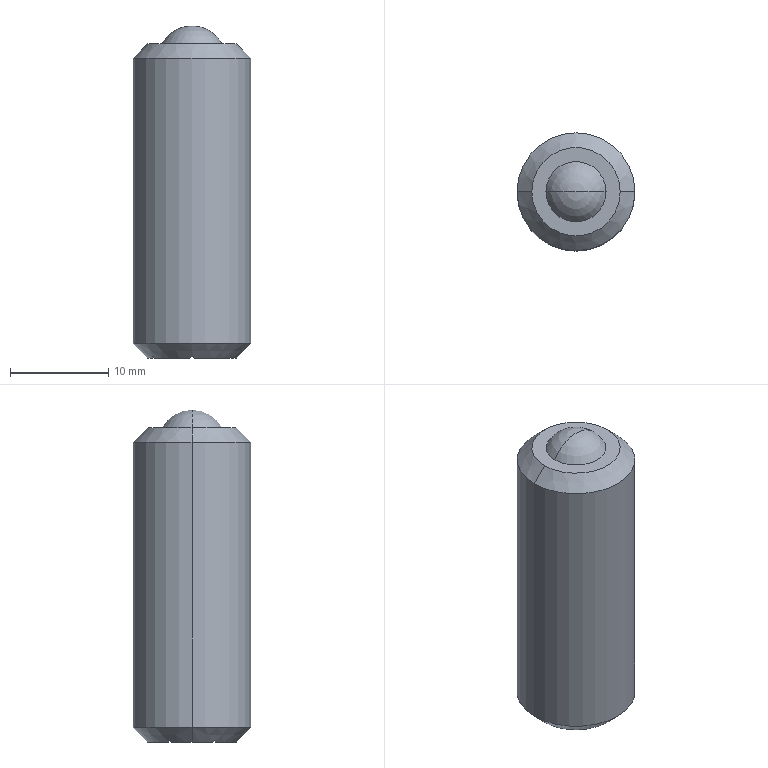Part | Creo | 1 solid | 22 faces | box 12 x 12 x 33.8 mm | volume 2573 mm3 | plane 14 | cone 4 | cylinder 2 | sphere 2 | commonest cylinder face diameters 12 x2
STEP:
#1=CARTESIAN_POINT('',(99.,-277.938,-72.5));
#2=VERTEX_POINT('',#1);
#3=CARTESIAN_POINT('',(99.,-282.062,-72.5));
#4=VERTEX_POINT('',#3);
#5=CARTESIAN_POINT('',(99.,-277.938,-72.5));
#6=DIRECTION('',(0.,-1.,0.));
#7=VECTOR('',#6,4.123);
#8=LINE('',#5,#7);
#9=EDGE_CURVE('',#2,#4,#8,.T.);
#10=ORIENTED_EDGE('',*,*,#9,.T.);
#11=CARTESIAN_POINT('',(99.5,-280.,-72.5));
#12=VERTEX_POINT('',#11);
#13=CARTESIAN_POINT('',(95.,-280.,-72.5));
#14=DIRECTION('',(0.,0.,-1.));
#15=DIRECTION('',(1.,0.,0.));
#16=AXIS2_PLACEMENT_3D('',#13,#14,#15);
#17=CIRCLE('',#16,4.5);
#18=EDGE_CURVE('',#12,#4,#17,.T.);
#19=ORIENTED_EDGE('',*,*,#18,.F.);
#20=CARTESIAN_POINT('',(95.,-280.,-72.5));
#21=DIRECTION('',(0.,0.,-1.));
#22=DIRECTION('',(0.8889,0.4581,0.));
#23=AXIS2_PLACEMENT_3D('',#20,#21,#22);
#24=CIRCLE('',#23,4.5);
#25=EDGE_CURVE('',#2,#12,#24,.T.);
#26=ORIENTED_EDGE('',*,*,#25,.F.);
#27=EDGE_LOOP('',(#10,#19,#26));
#28=FACE_OUTER_BOUND('',#27,.F.);
#29=CARTESIAN_POINT('',(95.,-280.,-72.5));
#30=DIRECTION('',(0.,0.,-1.));
#31=DIRECTION('',(-1.,0.,0.));
#32=AXIS2_PLACEMENT_3D('',#29,#30,#31);
#33=PLANE('',#32);
#34=ADVANCED_FACE('',(#28),#33,.T.);
#35=ORIENTED_EDGE('',*,*,#9,.F.);
#36=CARTESIAN_POINT('',(99.,-277.691,-72.381));
#37=VERTEX_POINT('',#36);
#38=CARTESIAN_POINT('',(99.,-277.938,-72.5));
#39=CARTESIAN_POINT('',(99.,-277.911,-72.487));
#40=CARTESIAN_POINT('',(99.,-277.856,-72.462));
#41=CARTESIAN_POINT('',(99.,-277.773,-72.422));
#42=CARTESIAN_POINT('',(99.,-277.718,-72.395));
#43=CARTESIAN_POINT('',(99.,-277.691,-72.381));
#44=B_SPLINE_CURVE_WITH_KNOTS('',3,(#38,#39,#40,#41,#42,#43),.UNSPECIFIED.,.F.,.F.,(4,1,1,4),(0.,0.3333,0.6667,1.),.UNSPECIFIED.);
#45=EDGE_CURVE('',#2,#37,#44,.T.);
#46=ORIENTED_EDGE('',*,*,#45,.T.);
#47=CARTESIAN_POINT('',(99.,-277.691,-54.5));
#48=VERTEX_POINT('',#47);
#49=CARTESIAN_POINT('',(99.,-277.691,-54.5));
#50=DIRECTION('',(0.,0.,-1.));
#51=VECTOR('',#50,17.881);
#52=LINE('',#49,#51);
#53=EDGE_CURVE('',#48,#37,#52,.T.);
#54=ORIENTED_EDGE('',*,*,#53,.F.);
#55=CARTESIAN_POINT('',(99.,-282.309,-54.5));
#56=VERTEX_POINT('',#55);
#57=CARTESIAN_POINT('',(99.,-277.691,-54.5));
#58=DIRECTION('',(0.,-1.,0.));
#59=VECTOR('',#58,4.619);
#60=LINE('',#57,#59);
#61=EDGE_CURVE('',#48,#56,#60,.T.);
#62=ORIENTED_EDGE('',*,*,#61,.T.);
#63=CARTESIAN_POINT('',(99.,-282.309,-72.381));
#64=VERTEX_POINT('',#63);
#65=CARTESIAN_POINT('',(99.,-282.309,-54.5));
#66=DIRECTION('',(0.,0.,-1.));
#67=VECTOR('',#66,17.881);
#68=LINE('',#65,#67);
#69=EDGE_CURVE('',#56,#64,#68,.T.);
#70=ORIENTED_EDGE('',*,*,#69,.T.);
#71=CARTESIAN_POINT('',(99.,-282.309,-72.381));
#72=CARTESIAN_POINT('',(99.,-282.282,-72.395));
#73=CARTESIAN_POINT('',(99.,-282.227,-72.422));
#74=CARTESIAN_POINT('',(99.,-282.144,-72.462));
#75=CARTESIAN_POINT('',(99.,-282.089,-72.487));
#76=CARTESIAN_POINT('',(99.,-282.062,-72.5));
#77=B_SPLINE_CURVE_WITH_KNOTS('',3,(#71,#72,#73,#74,#75,#76),.UNSPECIFIED.,.F.,.F.,(4,1,1,4),(0.,0.3333,0.6667,1.),.UNSPECIFIED.);
#78=EDGE_CURVE('',#64,#4,#77,.T.);
#79=ORIENTED_EDGE('',*,*,#78,.T.);
#80=EDGE_LOOP('',(#35,#46,#54,#62,#70,#79));
#81=FACE_OUTER_BOUND('',#80,.F.);
#82=CARTESIAN_POINT('',(99.,-280.,-68.5));
#83=DIRECTION('',(1.,0.,0.));
#84=DIRECTION('',(0.,0.,-1.));
#85=AXIS2_PLACEMENT_3D('',#82,#83,#84);
#86=PLANE('',#85);
#87=ADVANCED_FACE('',(#81),#86,.F.);
#88=ORIENTED_EDGE('',*,*,#25,.T.);
#89=CARTESIAN_POINT('',(101.,-280.,-71.));
#90=VERTEX_POINT('',#89);
#91=CARTESIAN_POINT('',(99.5,-280.,-72.5));
#92=DIRECTION('',(0.7071,0.,0.7071));
#93=VECTOR('',#92,2.121);
#94=LINE('',#91,#93);
#95=EDGE_CURVE('',#12,#90,#94,.T.);
#96=ORIENTED_EDGE('',*,*,#95,.T.);
#97=CARTESIAN_POINT('',(89.,-280.,-71.));
#98=VERTEX_POINT('',#97);
#99=CARTESIAN_POINT('',(95.,-280.,-71.));
#100=DIRECTION('',(0.,0.,-1.));
#101=DIRECTION('',(-1.,0.,0.));
#102=AXIS2_PLACEMENT_3D('',#99,#100,#101);
#103=CIRCLE('',#102,6.);
#104=EDGE_CURVE('',#98,#90,#103,.T.);
#105=ORIENTED_EDGE('',*,*,#104,.F.);
#106=CARTESIAN_POINT('',(90.5,-280.,-72.5));
#107=VERTEX_POINT('',#106);
#108=CARTESIAN_POINT('',(90.5,-280.,-72.5));
#109=DIRECTION('',(-0.7071,0.,0.7071));
#110=VECTOR('',#109,2.121);
#111=LINE('',#108,#110);
#112=EDGE_CURVE('',#107,#98,#111,.T.);
#113=ORIENTED_EDGE('',*,*,#112,.F.);
#114=CARTESIAN_POINT('',(91.,-277.938,-72.5));
#115=VERTEX_POINT('',#114);
#116=CARTESIAN_POINT('',(95.,-280.,-72.5));
#117=DIRECTION('',(0.,0.,-1.));
#118=DIRECTION('',(-1.,0.,0.));
#119=AXIS2_PLACEMENT_3D('',#116,#117,#118);
#120=CIRCLE('',#119,4.5);
#121=EDGE_CURVE('',#107,#115,#120,.T.);
#122=ORIENTED_EDGE('',*,*,#121,.T.);
#123=CARTESIAN_POINT('',(91.,-277.691,-72.381));
#124=VERTEX_POINT('',#123);
#125=CARTESIAN_POINT('',(91.,-277.691,-72.381));
#126=CARTESIAN_POINT('',(91.,-277.718,-72.395));
#127=CARTESIAN_POINT('',(91.,-277.773,-72.422));
#128=CARTESIAN_POINT('',(91.,-277.856,-72.462));
#129=CARTESIAN_POINT('',(91.,-277.911,-72.487));
#130=CARTESIAN_POINT('',(91.,-277.938,-72.5));
#131=B_SPLINE_CURVE_WITH_KNOTS('',3,(#125,#126,#127,#128,#129,#130),.UNSPECIFIED.,.F.,.F.,(4,1,1,4),(0.,0.3333,0.6667,1.),.UNSPECIFIED.);
#132=EDGE_CURVE('',#124,#115,#131,.T.);
#133=ORIENTED_EDGE('',*,*,#132,.F.);
#134=CARTESIAN_POINT('',(91.215,-277.567,-72.5));
#135=VERTEX_POINT('',#134);
#136=CARTESIAN_POINT('',(91.215,-277.567,-72.5));
#137=CARTESIAN_POINT('',(91.191,-277.58,-72.487));
#138=CARTESIAN_POINT('',(91.143,-277.608,-72.462));
#139=CARTESIAN_POINT('',(91.071,-277.649,-72.422));
#140=CARTESIAN_POINT('',(91.024,-277.677,-72.395));
#141=CARTESIAN_POINT('',(91.,-277.691,-72.381));
#142=B_SPLINE_CURVE_WITH_KNOTS('',3,(#136,#137,#138,#139,#140,#141),.UNSPECIFIED.,.F.,.F.,(4,1,1,4),(0.,0.3333,0.6667,1.),.UNSPECIFIED.);
#143=EDGE_CURVE('',#135,#124,#142,.T.);
#144=ORIENTED_EDGE('',*,*,#143,.F.);
#145=CARTESIAN_POINT('',(94.785,-275.505,-72.5));
#146=VERTEX_POINT('',#145);
#147=CARTESIAN_POINT('',(95.,-280.,-72.5));
#148=DIRECTION('',(0.,0.,-1.));
#149=DIRECTION('',(-0.8412,0.5407,0.));
#150=AXIS2_PLACEMENT_3D('',#147,#148,#149);
#151=CIRCLE('',#150,4.5);
#152=EDGE_CURVE('',#135,#146,#151,.T.);
#153=ORIENTED_EDGE('',*,*,#152,.T.);
#154=CARTESIAN_POINT('',(95.,-275.381,-72.381));
#155=VERTEX_POINT('',#154);
#156=CARTESIAN_POINT('',(95.,-275.381,-72.381));
#157=CARTESIAN_POINT('',(94.976,-275.395,-72.395));
#158=CARTESIAN_POINT('',(94.929,-275.422,-72.422));
#159=CARTESIAN_POINT('',(94.857,-275.464,-72.462));
#160=CARTESIAN_POINT('',(94.809,-275.491,-72.487));
#161=CARTESIAN_POINT('',(94.785,-275.505,-72.5));
#162=B_SPLINE_CURVE_WITH_KNOTS('',3,(#156,#157,#158,#159,#160,#161),.UNSPECIFIED.,.F.,.F.,(4,1,1,4),(0.,0.3333,0.6667,1.),.UNSPECIFIED.);
#163=EDGE_CURVE('',#155,#146,#162,.T.);
#164=ORIENTED_EDGE('',*,*,#163,.F.);
#165=CARTESIAN_POINT('',(95.215,-275.505,-72.5));
#166=VERTEX_POINT('',#165);
#167=CARTESIAN_POINT('',(95.215,-275.505,-72.5));
#168=CARTESIAN_POINT('',(95.191,-275.491,-72.487));
#169=CARTESIAN_POINT('',(95.143,-275.464,-72.462));
#170=CARTESIAN_POINT('',(95.071,-275.422,-72.422));
#171=CARTESIAN_POINT('',(95.024,-275.395,-72.395));
#172=CARTESIAN_POINT('',(95.,-275.381,-72.381));
#173=B_SPLINE_CURVE_WITH_KNOTS('',3,(#167,#168,#169,#170,#171,#172),.UNSPECIFIED.,.F.,.F.,(4,1,1,4),(0.,0.3333,0.6667,1.),.UNSPECIFIED.);
#174=EDGE_CURVE('',#166,#155,#173,.T.);
#175=ORIENTED_EDGE('',*,*,#174,.F.);
#176=CARTESIAN_POINT('',(98.785,-277.567,-72.5));
#177=VERTEX_POINT('',#176);
#178=CARTESIAN_POINT('',(95.,-280.,-72.5));
#179=DIRECTION('',(0.,0.,-1.));
#180=DIRECTION('',(0.0477,0.9989,0.));
#181=AXIS2_PLACEMENT_3D('',#178,#179,#180);
#182=CIRCLE('',#181,4.5);
#183=EDGE_CURVE('',#166,#177,#182,.T.);
#184=ORIENTED_EDGE('',*,*,#183,.T.);
#185=CARTESIAN_POINT('',(99.,-277.691,-72.381));
#186=CARTESIAN_POINT('',(98.976,-277.677,-72.395));
#187=CARTESIAN_POINT('',(98.929,-277.649,-72.422));
#188=CARTESIAN_POINT('',(98.857,-277.608,-72.462));
#189=CARTESIAN_POINT('',(98.809,-277.58,-72.487));
#190=CARTESIAN_POINT('',(98.785,-277.567,-72.5));
#191=B_SPLINE_CURVE_WITH_KNOTS('',3,(#185,#186,#187,#188,#189,#190),.UNSPECIFIED.,.F.,.F.,(4,1,1,4),(0.,0.3333,0.6667,1.),.UNSPECIFIED.);
#192=EDGE_CURVE('',#37,#177,#191,.T.);
#193=ORIENTED_EDGE('',*,*,#192,.F.);
#194=ORIENTED_EDGE('',*,*,#45,.F.);
#195=EDGE_LOOP('',(#88,#96,#105,#113,#122,#133,#144,#153,#164,#175,#184,#193,#194));
#196=FACE_OUTER_BOUND('',#195,.F.);
#197=CARTESIAN_POINT('',(95.,-280.,-71.75));
#198=DIRECTION('',(0.,0.,1.));
#199=DIRECTION('',(1.,0.,0.));
#200=AXIS2_PLACEMENT_3D('',#197,#198,#199);
#201=CONICAL_SURFACE('',#200,5.25,45.);
#202=ADVANCED_FACE('',(#196),#201,.T.);
#203=ORIENTED_EDGE('',*,*,#78,.F.);
#204=CARTESIAN_POINT('',(98.785,-282.433,-72.5));
#205=VERTEX_POINT('',#204);
#206=CARTESIAN_POINT('',(98.785,-282.433,-72.5));
#207=CARTESIAN_POINT('',(98.809,-282.42,-72.487));
#208=CARTESIAN_POINT('',(98.857,-282.392,-72.462));
#209=CARTESIAN_POINT('',(98.929,-282.351,-72.422));
#210=CARTESIAN_POINT('',(98.976,-282.323,-72.395));
#211=CARTESIAN_POINT('',(99.,-282.309,-72.381));
#212=B_SPLINE_CURVE_WITH_KNOTS('',3,(#206,#207,#208,#209,#210,#211),.UNSPECIFIED.,.F.,.F.,(4,1,1,4),(0.,0.3333,0.6667,1.),.UNSPECIFIED.);
#213=EDGE_CURVE('',#205,#64,#212,.T.);
#214=ORIENTED_EDGE('',*,*,#213,.F.);
#215=CARTESIAN_POINT('',(95.215,-284.495,-72.5));
#216=VERTEX_POINT('',#215);
#217=CARTESIAN_POINT('',(95.,-280.,-72.5));
#218=DIRECTION('',(0.,0.,-1.));
#219=DIRECTION('',(0.8412,-0.5407,0.));
#220=AXIS2_PLACEMENT_3D('',#217,#218,#219);
#221=CIRCLE('',#220,4.5);
#222=EDGE_CURVE('',#205,#216,#221,.T.);
#223=ORIENTED_EDGE('',*,*,#222,.T.);
#224=CARTESIAN_POINT('',(95.,-284.619,-72.381));
#225=VERTEX_POINT('',#224);
#226=CARTESIAN_POINT('',(95.,-284.619,-72.381));
#227=CARTESIAN_POINT('',(95.024,-284.605,-72.395));
#228=CARTESIAN_POINT('',(95.071,-284.578,-72.422));
#229=CARTESIAN_POINT('',(95.143,-284.536,-72.462));
#230=CARTESIAN_POINT('',(95.191,-284.509,-72.487));
#231=CARTESIAN_POINT('',(95.215,-284.495,-72.5));
#232=B_SPLINE_CURVE_WITH_KNOTS('',3,(#226,#227,#228,#229,#230,#231),.UNSPECIFIED.,.F.,.F.,(4,1,1,4),(0.,0.3333,0.6667,1.),.UNSPECIFIED.);
#233=EDGE_CURVE('',#225,#216,#232,.T.);
#234=ORIENTED_EDGE('',*,*,#233,.F.);
#235=CARTESIAN_POINT('',(94.785,-284.495,-72.5));
#236=VERTEX_POINT('',#235);
#237=CARTESIAN_POINT('',(94.785,-284.495,-72.5));
#238=CARTESIAN_POINT('',(94.809,-284.509,-72.487));
#239=CARTESIAN_POINT('',(94.857,-284.536,-72.462));
#240=CARTESIAN_POINT('',(94.929,-284.578,-72.422));
#241=CARTESIAN_POINT('',(94.976,-284.605,-72.395));
#242=CARTESIAN_POINT('',(95.,-284.619,-72.381));
#243=B_SPLINE_CURVE_WITH_KNOTS('',3,(#237,#238,#239,#240,#241,#242),.UNSPECIFIED.,.F.,.F.,(4,1,1,4),(0.,0.3333,0.6667,1.),.UNSPECIFIED.);
#244=EDGE_CURVE('',#236,#225,#243,.T.);
#245=ORIENTED_EDGE('',*,*,#244,.F.);
#246=CARTESIAN_POINT('',(91.215,-282.433,-72.5));
#247=VERTEX_POINT('',#246);
#248=CARTESIAN_POINT('',(95.,-280.,-72.5));
#249=DIRECTION('',(0.,0.,-1.));
#250=DIRECTION('',(-0.0477,-0.9989,0.));
#251=AXIS2_PLACEMENT_3D('',#248,#249,#250);
#252=CIRCLE('',#251,4.5);
#253=EDGE_CURVE('',#236,#247,#252,.T.);
#254=ORIENTED_EDGE('',*,*,#253,.T.);
#255=CARTESIAN_POINT('',(91.,-282.309,-72.381));
#256=VERTEX_POINT('',#255);
#257=CARTESIAN_POINT('',(91.,-282.309,-72.381));
#258=CARTESIAN_POINT('',(91.024,-282.323,-72.395));
#259=CARTESIAN_POINT('',(91.071,-282.351,-72.422));
#260=CARTESIAN_POINT('',(91.143,-282.392,-72.462));
#261=CARTESIAN_POINT('',(91.191,-282.42,-72.487));
#262=CARTESIAN_POINT('',(91.215,-282.433,-72.5));
#263=B_SPLINE_CURVE_WITH_KNOTS('',3,(#257,#258,#259,#260,#261,#262),.UNSPECIFIED.,.F.,.F.,(4,1,1,4),(0.,0.3333,0.6667,1.),.UNSPECIFIED.);
#264=EDGE_CURVE('',#256,#247,#263,.T.);
#265=ORIENTED_EDGE('',*,*,#264,.F.);
#266=CARTESIAN_POINT('',(91.,-282.062,-72.5));
#267=VERTEX_POINT('',#266);
#268=CARTESIAN_POINT('',(91.,-282.062,-72.5));
#269=CARTESIAN_POINT('',(91.,-282.089,-72.487));
#270=CARTESIAN_POINT('',(91.,-282.144,-72.462));
#271=CARTESIAN_POINT('',(91.,-282.227,-72.422));
#272=CARTESIAN_POINT('',(91.,-282.282,-72.395));
#273=CARTESIAN_POINT('',(91.,-282.309,-72.381));
#274=B_SPLINE_CURVE_WITH_KNOTS('',3,(#268,#269,#270,#271,#272,#273),.UNSPECIFIED.,.F.,.F.,(4,1,1,4),(0.,0.3333,0.6667,1.),.UNSPECIFIED.);
#275=EDGE_CURVE('',#267,#256,#274,.T.);
#276=ORIENTED_EDGE('',*,*,#275,.F.);
#277=CARTESIAN_POINT('',(95.,-280.,-72.5));
#278=DIRECTION('',(0.,0.,-1.));
#279=DIRECTION('',(-0.8889,-0.4581,0.));
#280=AXIS2_PLACEMENT_3D('',#277,#278,#279);
#281=CIRCLE('',#280,4.5);
#282=EDGE_CURVE('',#267,#107,#281,.T.);
#283=ORIENTED_EDGE('',*,*,#282,.T.);
#284=ORIENTED_EDGE('',*,*,#112,.T.);
#285=CARTESIAN_POINT('',(95.,-280.,-71.));
#286=DIRECTION('',(0.,0.,-1.));
#287=DIRECTION('',(1.,0.,0.));
#288=AXIS2_PLACEMENT_3D('',#285,#286,#287);
#289=CIRCLE('',#288,6.);
#290=EDGE_CURVE('',#90,#98,#289,.T.);
#291=ORIENTED_EDGE('',*,*,#290,.F.);
#292=ORIENTED_EDGE('',*,*,#95,.F.);
#293=ORIENTED_EDGE('',*,*,#18,.T.);
#294=EDGE_LOOP('',(#203,#214,#223,#234,#245,#254,#265,#276,#283,#284,#291,#292,#293));
#295=FACE_OUTER_BOUND('',#294,.F.);
#296=CARTESIAN_POINT('',(95.,-280.,-71.75));
#297=DIRECTION('',(0.,0.,1.));
#298=DIRECTION('',(1.,0.,0.));
#299=AXIS2_PLACEMENT_3D('',#296,#297,#298);
#300=CONICAL_SURFACE('',#299,5.25,45.);
#301=ADVANCED_FACE('',(#295),#300,.T.);
#302=ORIENTED_EDGE('',*,*,#69,.F.);
#303=CARTESIAN_POINT('',(95.,-284.619,-54.5));
#304=VERTEX_POINT('',#303);
#305=CARTESIAN_POINT('',(99.,-282.309,-54.5));
#306=DIRECTION('',(-0.866,-0.5,0.));
#307=VECTOR('',#306,4.619);
#308=LINE('',#305,#307);
#309=EDGE_CURVE('',#56,#304,#308,.T.);
#310=ORIENTED_EDGE('',*,*,#309,.T.);
#311=CARTESIAN_POINT('',(95.,-284.619,-54.5));
#312=DIRECTION('',(0.,0.,-1.));
#313=VECTOR('',#312,17.881);
#314=LINE('',#311,#313);
#315=EDGE_CURVE('',#304,#225,#314,.T.);
#316=ORIENTED_EDGE('',*,*,#315,.T.);
#317=ORIENTED_EDGE('',*,*,#233,.T.);
#318=CARTESIAN_POINT('',(95.215,-284.495,-72.5));
#319=DIRECTION('',(0.866,0.5,0.));
#320=VECTOR('',#319,4.123);
#321=LINE('',#318,#320);
#322=EDGE_CURVE('',#216,#205,#321,.T.);
#323=ORIENTED_EDGE('',*,*,#322,.T.);
#324=ORIENTED_EDGE('',*,*,#213,.T.);
#325=EDGE_LOOP('',(#302,#310,#316,#317,#323,#324));
#326=FACE_OUTER_BOUND('',#325,.F.);
#327=CARTESIAN_POINT('',(97.,-283.464,-68.5));
#328=DIRECTION('',(0.5,-0.866,0.));
#329=DIRECTION('',(0.866,0.5,0.));
#330=AXIS2_PLACEMENT_3D('',#327,#328,#329);
#331=PLANE('',#330);
#332=ADVANCED_FACE('',(#326),#331,.F.);
#333=CARTESIAN_POINT('',(91.,-282.309,-54.5));
#334=VERTEX_POINT('',#333);
#335=CARTESIAN_POINT('',(91.,-277.691,-54.5));
#336=VERTEX_POINT('',#335);
#337=CARTESIAN_POINT('',(91.,-282.309,-54.5));
#338=DIRECTION('',(0.,1.,0.));
#339=VECTOR('',#338,4.619);
#340=LINE('',#337,#339);
#341=EDGE_CURVE('',#334,#336,#340,.T.);
#342=ORIENTED_EDGE('',*,*,#341,.F.);
#343=CARTESIAN_POINT('',(95.,-284.619,-54.5));
#344=DIRECTION('',(-0.866,0.5,0.));
#345=VECTOR('',#344,4.619);
#346=LINE('',#343,#345);
#347=EDGE_CURVE('',#304,#334,#346,.T.);
#348=ORIENTED_EDGE('',*,*,#347,.F.);
#349=ORIENTED_EDGE('',*,*,#309,.F.);
#350=ORIENTED_EDGE('',*,*,#61,.F.);
#351=CARTESIAN_POINT('',(95.,-275.381,-54.5));
#352=VERTEX_POINT('',#351);
#353=CARTESIAN_POINT('',(95.,-275.381,-54.5));
#354=DIRECTION('',(0.866,-0.5,0.));
#355=VECTOR('',#354,4.619);
#356=LINE('',#353,#355);
#357=EDGE_CURVE('',#352,#48,#356,.T.);
#358=ORIENTED_EDGE('',*,*,#357,.F.);
#359=CARTESIAN_POINT('',(91.,-277.691,-54.5));
#360=DIRECTION('',(0.866,0.5,0.));
#361=VECTOR('',#360,4.619);
#362=LINE('',#359,#361);
#363=EDGE_CURVE('',#336,#352,#362,.T.);
#364=ORIENTED_EDGE('',*,*,#363,.F.);
#365=EDGE_LOOP('',(#342,#348,#349,#350,#358,#364));
#366=FACE_OUTER_BOUND('',#365,.F.);
#367=CARTESIAN_POINT('',(95.,-280.,-54.5));
#368=DIRECTION('',(0.,0.,1.));
#369=DIRECTION('',(1.,0.,0.));
#370=AXIS2_PLACEMENT_3D('',#367,#368,#369);
#371=PLANE('',#370);
#372=ADVANCED_FACE('',(#366),#371,.F.);
#373=CARTESIAN_POINT('',(91.,-282.309,-54.5));
#374=DIRECTION('',(0.,0.,-1.));
#375=VECTOR('',#374,17.881);
#376=LINE('',#373,#375);
#377=EDGE_CURVE('',#334,#256,#376,.T.);
#378=ORIENTED_EDGE('',*,*,#377,.F.);
#379=ORIENTED_EDGE('',*,*,#341,.T.);
#380=CARTESIAN_POINT('',(91.,-277.691,-54.5));
#381=DIRECTION('',(0.,0.,-1.));
#382=VECTOR('',#381,17.881);
#383=LINE('',#380,#382);
#384=EDGE_CURVE('',#336,#124,#383,.T.);
#385=ORIENTED_EDGE('',*,*,#384,.T.);
#386=ORIENTED_EDGE('',*,*,#132,.T.);
#387=CARTESIAN_POINT('',(91.,-282.062,-72.5));
#388=DIRECTION('',(0.,1.,0.));
#389=VECTOR('',#388,4.123);
#390=LINE('',#387,#389);
#391=EDGE_CURVE('',#267,#115,#390,.T.);
#392=ORIENTED_EDGE('',*,*,#391,.F.);
#393=ORIENTED_EDGE('',*,*,#275,.T.);
#394=EDGE_LOOP('',(#378,#379,#385,#386,#392,#393));
#395=FACE_OUTER_BOUND('',#394,.F.);
#396=CARTESIAN_POINT('',(91.,-280.,-68.5));
#397=DIRECTION('',(-1.,0.,0.));
#398=DIRECTION('',(0.,0.,1.));
#399=AXIS2_PLACEMENT_3D('',#396,#397,#398);
#400=PLANE('',#399);
#401=ADVANCED_FACE('',(#395),#400,.F.);
#402=ORIENTED_EDGE('',*,*,#315,.F.);
#403=ORIENTED_EDGE('',*,*,#347,.T.);
#404=ORIENTED_EDGE('',*,*,#377,.T.);
#405=ORIENTED_EDGE('',*,*,#264,.T.);
#406=CARTESIAN_POINT('',(91.215,-282.433,-72.5));
#407=DIRECTION('',(0.866,-0.5,0.));
#408=VECTOR('',#407,4.123);
#409=LINE('',#406,#408);
#410=EDGE_CURVE('',#247,#236,#409,.T.);
#411=ORIENTED_EDGE('',*,*,#410,.T.);
#412=ORIENTED_EDGE('',*,*,#244,.T.);
#413=EDGE_LOOP('',(#402,#403,#404,#405,#411,#412));
#414=FACE_OUTER_BOUND('',#413,.F.);
#415=CARTESIAN_POINT('',(93.,-283.464,-68.5));
#416=DIRECTION('',(-0.5,-0.866,0.));
#417=DIRECTION('',(0.866,-0.5,0.));
#418=AXIS2_PLACEMENT_3D('',#415,#416,#417);
#419=PLANE('',#418);
#420=ADVANCED_FACE('',(#414),#419,.F.);
#421=ORIENTED_EDGE('',*,*,#410,.F.);
#422=ORIENTED_EDGE('',*,*,#253,.F.);
#423=EDGE_LOOP('',(#421,#422));
#424=FACE_OUTER_BOUND('',#423,.F.);
#425=CARTESIAN_POINT('',(75.,-280.,-72.5));
#426=DIRECTION('',(0.,0.,-1.));
#427=DIRECTION('',(-1.,0.,0.));
#428=AXIS2_PLACEMENT_3D('',#425,#426,#427);
#429=PLANE('',#428);
#430=ADVANCED_FACE('',(#424),#429,.T.);
#431=ORIENTED_EDGE('',*,*,#384,.F.);
#432=ORIENTED_EDGE('',*,*,#363,.T.);
#433=CARTESIAN_POINT('',(95.,-275.381,-54.5));
#434=DIRECTION('',(0.,0.,-1.));
#435=VECTOR('',#434,17.881);
#436=LINE('',#433,#435);
#437=EDGE_CURVE('',#352,#155,#436,.T.);
#438=ORIENTED_EDGE('',*,*,#437,.T.);
#439=ORIENTED_EDGE('',*,*,#163,.T.);
#440=CARTESIAN_POINT('',(94.785,-275.505,-72.5));
#441=DIRECTION('',(-0.866,-0.5,0.));
#442=VECTOR('',#441,4.123);
#443=LINE('',#440,#442);
#444=EDGE_CURVE('',#146,#135,#443,.T.);
#445=ORIENTED_EDGE('',*,*,#444,.T.);
#446=ORIENTED_EDGE('',*,*,#143,.T.);
#447=EDGE_LOOP('',(#431,#432,#438,#439,#445,#446));
#448=FACE_OUTER_BOUND('',#447,.F.);
#449=CARTESIAN_POINT('',(93.,-276.536,-68.5));
#450=DIRECTION('',(-0.5,0.866,0.));
#451=DIRECTION('',(-0.866,-0.5,0.));
#452=AXIS2_PLACEMENT_3D('',#449,#450,#451);
#453=PLANE('',#452);
#454=ADVANCED_FACE('',(#448),#453,.F.);
#455=ORIENTED_EDGE('',*,*,#437,.F.);
#456=ORIENTED_EDGE('',*,*,#357,.T.);
#457=ORIENTED_EDGE('',*,*,#53,.T.);
#458=ORIENTED_EDGE('',*,*,#192,.T.);
#459=CARTESIAN_POINT('',(98.785,-277.567,-72.5));
#460=DIRECTION('',(-0.866,0.5,0.));
#461=VECTOR('',#460,4.123);
#462=LINE('',#459,#461);
#463=EDGE_CURVE('',#177,#166,#462,.T.);
#464=ORIENTED_EDGE('',*,*,#463,.T.);
#465=ORIENTED_EDGE('',*,*,#174,.T.);
#466=EDGE_LOOP('',(#455,#456,#457,#458,#464,#465));
#467=FACE_OUTER_BOUND('',#466,.F.);
#468=CARTESIAN_POINT('',(97.,-276.536,-68.5));
#469=DIRECTION('',(0.5,0.866,0.));
#470=DIRECTION('',(-0.866,0.5,0.));
#471=AXIS2_PLACEMENT_3D('',#468,#469,#470);
#472=PLANE('',#471);
#473=ADVANCED_FACE('',(#467),#472,.F.);
#474=ORIENTED_EDGE('',*,*,#463,.F.);
#475=ORIENTED_EDGE('',*,*,#183,.F.);
#476=EDGE_LOOP('',(#474,#475));
#477=FACE_OUTER_BOUND('',#476,.F.);
#478=CARTESIAN_POINT('',(95.,-280.,-72.5));
#479=DIRECTION('',(0.,0.,-1.));
#480=DIRECTION('',(-1.,0.,0.));
#481=AXIS2_PLACEMENT_3D('',#478,#479,#480);
#482=PLANE('',#481);
#483=ADVANCED_FACE('',(#477),#482,.T.);
#484=ORIENTED_EDGE('',*,*,#444,.F.);
#485=ORIENTED_EDGE('',*,*,#152,.F.);
#486=EDGE_LOOP('',(#484,#485));
#487=FACE_OUTER_BOUND('',#486,.F.);
#488=CARTESIAN_POINT('',(95.,-280.,-72.5));
#489=DIRECTION('',(0.,0.,-1.));
#490=DIRECTION('',(-1.,0.,0.));
#491=AXIS2_PLACEMENT_3D('',#488,#489,#490);
#492=PLANE('',#491);
#493=ADVANCED_FACE('',(#487),#492,.T.);
#494=ORIENTED_EDGE('',*,*,#121,.F.);
#495=ORIENTED_EDGE('',*,*,#282,.F.);
#496=ORIENTED_EDGE('',*,*,#391,.T.);
#497=EDGE_LOOP('',(#494,#495,#496));
#498=FACE_OUTER_BOUND('',#497,.F.);
#499=CARTESIAN_POINT('',(95.,-280.,-72.5));
#500=DIRECTION('',(0.,0.,-1.));
#501=DIRECTION('',(-1.,0.,0.));
#502=AXIS2_PLACEMENT_3D('',#499,#500,#501);
#503=PLANE('',#502);
#504=ADVANCED_FACE('',(#498),#503,.T.);
#505=ORIENTED_EDGE('',*,*,#322,.F.);
#506=ORIENTED_EDGE('',*,*,#222,.F.);
#507=EDGE_LOOP('',(#505,#506));
#508=FACE_OUTER_BOUND('',#507,.F.);
#509=CARTESIAN_POINT('',(75.,-280.,-72.5));
#510=DIRECTION('',(0.,0.,-1.));
#511=DIRECTION('',(-1.,0.,0.));
#512=AXIS2_PLACEMENT_3D('',#509,#510,#511);
#513=PLANE('',#512);
#514=ADVANCED_FACE('',(#508),#513,.T.);
#515=ORIENTED_EDGE('',*,*,#290,.T.);
#516=CARTESIAN_POINT('',(89.,-280.,-42.));
#517=VERTEX_POINT('',#516);
#518=CARTESIAN_POINT('',(89.,-280.,-42.));
#519=DIRECTION('',(0.,0.,-1.));
#520=VECTOR('',#519,29.);
#521=LINE('',#518,#520);
#522=EDGE_CURVE('',#517,#98,#521,.T.);
#523=ORIENTED_EDGE('',*,*,#522,.F.);
#524=CARTESIAN_POINT('',(101.,-280.,-42.));
#525=VERTEX_POINT('',#524);
#526=CARTESIAN_POINT('',(95.,-280.,-42.));
#527=DIRECTION('',(0.,0.,1.));
#528=DIRECTION('',(-1.,0.,0.));
#529=AXIS2_PLACEMENT_3D('',#526,#527,#528);
#530=CIRCLE('',#529,6.);
#531=EDGE_CURVE('',#517,#525,#530,.T.);
#532=ORIENTED_EDGE('',*,*,#531,.T.);
#533=CARTESIAN_POINT('',(101.,-280.,-42.));
#534=DIRECTION('',(0.,0.,-1.));
#535=VECTOR('',#534,29.);
#536=LINE('',#533,#535);
#537=EDGE_CURVE('',#525,#90,#536,.T.);
#538=ORIENTED_EDGE('',*,*,#537,.T.);
#539=EDGE_LOOP('',(#515,#523,#532,#538));
#540=FACE_OUTER_BOUND('',#539,.F.);
#541=CARTESIAN_POINT('',(95.,-280.,-50.5));
#542=DIRECTION('',(0.,0.,-1.));
#543=DIRECTION('',(-1.,0.,0.));
#544=AXIS2_PLACEMENT_3D('',#541,#542,#543);
#545=CYLINDRICAL_SURFACE('',#544,6.);
#546=ADVANCED_FACE('',(#540),#545,.T.);
#547=ORIENTED_EDGE('',*,*,#104,.T.);
#548=ORIENTED_EDGE('',*,*,#537,.F.);
#549=CARTESIAN_POINT('',(95.,-280.,-42.));
#550=DIRECTION('',(0.,0.,1.));
#551=DIRECTION('',(1.,0.,0.));
#552=AXIS2_PLACEMENT_3D('',#549,#550,#551);
#553=CIRCLE('',#552,6.);
#554=EDGE_CURVE('',#525,#517,#553,.T.);
#555=ORIENTED_EDGE('',*,*,#554,.T.);
#556=ORIENTED_EDGE('',*,*,#522,.T.);
#557=EDGE_LOOP('',(#547,#548,#555,#556));
#558=FACE_OUTER_BOUND('',#557,.F.);
#559=CARTESIAN_POINT('',(95.,-280.,-50.5));
#560=DIRECTION('',(0.,0.,-1.));
#561=DIRECTION('',(-1.,0.,0.));
#562=AXIS2_PLACEMENT_3D('',#559,#560,#561);
#563=CYLINDRICAL_SURFACE('',#562,6.);
#564=ADVANCED_FACE('',(#558),#563,.T.);
#565=CARTESIAN_POINT('',(99.5,-280.,-40.5));
#566=VERTEX_POINT('',#565);
#567=CARTESIAN_POINT('',(90.5,-280.,-40.5));
#568=VERTEX_POINT('',#567);
#569=CARTESIAN_POINT('',(95.,-280.,-40.5));
#570=DIRECTION('',(0.,0.,1.));
#571=DIRECTION('',(1.,0.,0.));
#572=AXIS2_PLACEMENT_3D('',#569,#570,#571);
#573=CIRCLE('',#572,4.5);
#574=EDGE_CURVE('',#566,#568,#573,.T.);
#575=ORIENTED_EDGE('',*,*,#574,.T.);
#576=CARTESIAN_POINT('',(90.5,-280.,-40.5));
#577=DIRECTION('',(-0.7071,0.,-0.7071));
#578=VECTOR('',#577,2.121);
#579=LINE('',#576,#578);
#580=EDGE_CURVE('',#568,#517,#579,.T.);
#581=ORIENTED_EDGE('',*,*,#580,.T.);
#582=ORIENTED_EDGE('',*,*,#554,.F.);
#583=CARTESIAN_POINT('',(99.5,-280.,-40.5));
#584=DIRECTION('',(0.7071,0.,-0.7071));
#585=VECTOR('',#584,2.121);
#586=LINE('',#583,#585);
#587=EDGE_CURVE('',#566,#525,#586,.T.);
#588=ORIENTED_EDGE('',*,*,#587,.F.);
#589=EDGE_LOOP('',(#575,#581,#582,#588));
#590=FACE_OUTER_BOUND('',#589,.F.);
#591=CARTESIAN_POINT('',(95.,-280.,-41.25));
#592=DIRECTION('',(0.,0.,-1.));
#593=DIRECTION('',(-1.,0.,0.));
#594=AXIS2_PLACEMENT_3D('',#591,#592,#593);
#595=CONICAL_SURFACE('',#594,5.25,45.);
#596=ADVANCED_FACE('',(#590),#595,.T.);
#597=ORIENTED_EDGE('',*,*,#574,.F.);
#598=CARTESIAN_POINT('',(95.,-280.,-40.5));
#599=DIRECTION('',(0.,0.,1.));
#600=DIRECTION('',(-1.,0.,0.));
#601=AXIS2_PLACEMENT_3D('',#598,#599,#600);
#602=CIRCLE('',#601,4.5);
#603=EDGE_CURVE('',#568,#566,#602,.T.);
#604=ORIENTED_EDGE('',*,*,#603,.F.);
#605=EDGE_LOOP('',(#597,#604));
#606=FACE_OUTER_BOUND('',#605,.F.);
#607=CARTESIAN_POINT('',(98.059,-280.,-40.5));
#608=VERTEX_POINT('',#607);
#609=CARTESIAN_POINT('',(91.941,-280.,-40.5));
#610=VERTEX_POINT('',#609);
#611=CARTESIAN_POINT('',(95.,-280.,-40.5));
#612=DIRECTION('',(0.,0.,-1.));
#613=DIRECTION('',(1.,0.,0.));
#614=AXIS2_PLACEMENT_3D('',#611,#612,#613);
#615=CIRCLE('',#614,3.059);
#616=EDGE_CURVE('',#608,#610,#615,.T.);
#617=ORIENTED_EDGE('',*,*,#616,.F.);
#618=CARTESIAN_POINT('',(95.,-280.,-40.5));
#619=DIRECTION('',(0.,0.,-1.));
#620=DIRECTION('',(-1.,0.,0.));
#621=AXIS2_PLACEMENT_3D('',#618,#619,#620);
#622=CIRCLE('',#621,3.059);
#623=EDGE_CURVE('',#610,#608,#622,.T.);
#624=ORIENTED_EDGE('',*,*,#623,.F.);
#625=EDGE_LOOP('',(#617,#624));
#626=FACE_BOUND('',#625,.F.);
#627=CARTESIAN_POINT('',(95.,-280.,-40.5));
#628=DIRECTION('',(0.,0.,1.));
#629=DIRECTION('',(1.,0.,0.));
#630=AXIS2_PLACEMENT_3D('',#627,#628,#629);
#631=PLANE('',#630);
#632=ADVANCED_FACE('',(#606,#626),#631,.T.);
#633=ORIENTED_EDGE('',*,*,#616,.T.);
#634=CARTESIAN_POINT('',(95.,-280.,-38.7));
#635=VERTEX_POINT('',#634);
#636=CARTESIAN_POINT('',(95.,-280.,-42.2));
#637=DIRECTION('',(0.,1.,0.));
#638=DIRECTION('',(-0.8741,0.,0.4857));
#639=AXIS2_PLACEMENT_3D('',#636,#637,#638);
#640=CIRCLE('',#639,3.5);
#641=EDGE_CURVE('',#610,#635,#640,.T.);
#642=ORIENTED_EDGE('',*,*,#641,.T.);
#643=CARTESIAN_POINT('',(95.,-280.,-42.2));
#644=DIRECTION('',(0.,-1.,0.));
#645=DIRECTION('',(0.8741,0.,0.4857));
#646=AXIS2_PLACEMENT_3D('',#643,#644,#645);
#647=CIRCLE('',#646,3.5);
#648=EDGE_CURVE('',#608,#635,#647,.T.);
#649=ORIENTED_EDGE('',*,*,#648,.F.);
#650=EDGE_LOOP('',(#633,#642,#649));
#651=FACE_OUTER_BOUND('',#650,.F.);
#652=CARTESIAN_POINT('',(95.,-280.,-42.2));
#653=DIRECTION('',(0.,0.,1.));
#654=DIRECTION('',(1.,0.,0.));
#655=AXIS2_PLACEMENT_3D('',#652,#653,#654);
#656=SPHERICAL_SURFACE('',#655,3.5);
#657=ADVANCED_FACE('',(#651),#656,.T.);
#658=ORIENTED_EDGE('',*,*,#623,.T.);
#659=ORIENTED_EDGE('',*,*,#648,.T.);
#660=ORIENTED_EDGE('',*,*,#641,.F.);
#661=EDGE_LOOP('',(#658,#659,#660));
#662=FACE_OUTER_BOUND('',#661,.F.);
#663=CARTESIAN_POINT('',(95.,-280.,-42.2));
#664=DIRECTION('',(0.,0.,1.));
#665=DIRECTION('',(1.,0.,0.));
#666=AXIS2_PLACEMENT_3D('',#663,#664,#665);
#667=SPHERICAL_SURFACE('',#666,3.5);
#668=ADVANCED_FACE('',(#662),#667,.T.);
#669=ORIENTED_EDGE('',*,*,#603,.T.);
#670=ORIENTED_EDGE('',*,*,#587,.T.);
#671=ORIENTED_EDGE('',*,*,#531,.F.);
#672=ORIENTED_EDGE('',*,*,#580,.F.);
#673=EDGE_LOOP('',(#669,#670,#671,#672));
#674=FACE_OUTER_BOUND('',#673,.F.);
#675=CARTESIAN_POINT('',(95.,-280.,-41.25));
#676=DIRECTION('',(0.,0.,-1.));
#677=DIRECTION('',(-1.,0.,0.));
#678=AXIS2_PLACEMENT_3D('',#675,#676,#677);
#679=CONICAL_SURFACE('',#678,5.25,45.);
#680=ADVANCED_FACE('',(#674),#679,.T.);
#681=CLOSED_SHELL('',(#34,#87,#202,#301,#332,#372,#401,#420,#430,#454,#473,#483,#493,#504,#514,#546,#564,#596,#632,#657,#668,#680));
#682=MANIFOLD_SOLID_BREP('',#681);
#683=(LENGTH_UNIT()NAMED_UNIT(*)SI_UNIT(.MILLI.,.METRE.));
#684=UNCERTAINTY_MEASURE_WITH_UNIT(LENGTH_MEASURE(0.003782),#683,'','');
#685=(NAMED_UNIT(*)PLANE_ANGLE_UNIT()SI_UNIT($,.RADIAN.));
#686=PLANE_ANGLE_MEASURE_WITH_UNIT(PLANE_ANGLE_MEASURE(0.01745),#685);
#687=(CONVERSION_BASED_UNIT('DEGREE',#686)NAMED_UNIT(*)PLANE_ANGLE_UNIT());
#688=(NAMED_UNIT(*)SI_UNIT($,.STERADIAN.)SOLID_ANGLE_UNIT());
#689=(GEOMETRIC_REPRESENTATION_CONTEXT(3)GLOBAL_UNCERTAINTY_ASSIGNED_CONTEXT((#684))GLOBAL_UNIT_ASSIGNED_CONTEXT((#683,#687,#688))REPRESENTATION_CONTEXT('',''));
#690=ADVANCED_BREP_SHAPE_REPRESENTATION('',(#682),#689);